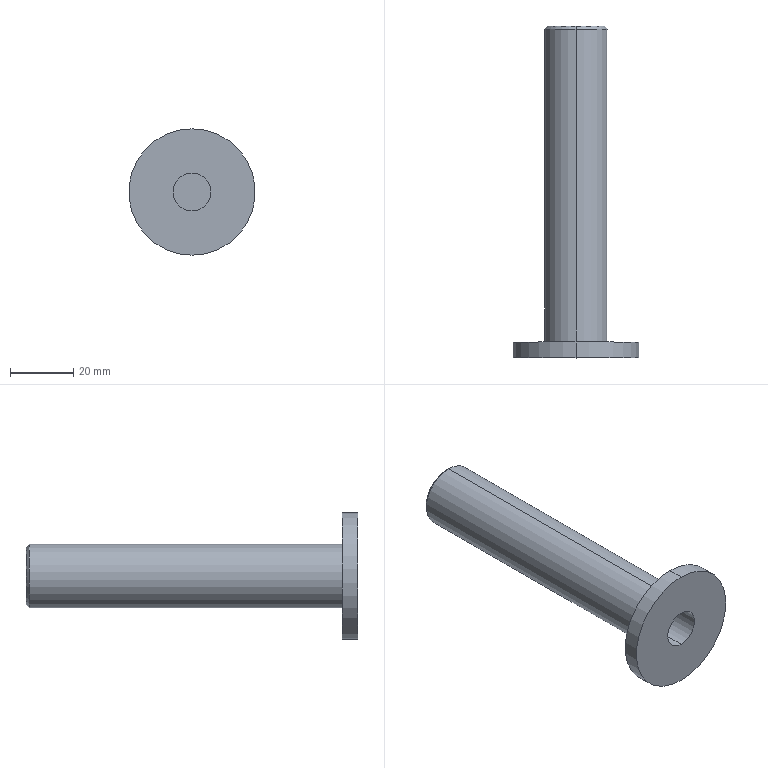Part | STEP file | Guide wheel mechanism revised.sldasm-Part-336 | 1 solid | 12 faces | box 40 x 105 x 40 mm | volume 36538 mm3 | cylinder 6 | plane 4 | cone 2 | commonest cylinder face diameters 12 x2 20 x2 40 x2
STEP:
#1=CARTESIAN_POINT('',(0.,10.,6.));
#2=VERTEX_POINT('',#1);
#3=CARTESIAN_POINT('',(0.,10.,-6.));
#4=VERTEX_POINT('',#3);
#5=CARTESIAN_POINT('',(0.,10.,0.));
#6=DIRECTION('',(0.,-1.,0.));
#7=DIRECTION('',(0.,0.,-1.));
#8=AXIS2_PLACEMENT_3D('',#5,#6,#7);
#9=CIRCLE('',#8,6.);
#10=EDGE_CURVE('',#2,#4,#9,.T.);
#11=ORIENTED_EDGE('',*,*,#10,.F.);
#12=CARTESIAN_POINT('',(0.,0.,6.));
#13=VERTEX_POINT('',#12);
#14=CARTESIAN_POINT('',(0.,10.,6.));
#15=DIRECTION('',(0.,-1.,0.));
#16=VECTOR('',#15,1000.);
#17=LINE('',#14,#16);
#18=EDGE_CURVE('',#2,#13,#17,.T.);
#19=ORIENTED_EDGE('',*,*,#18,.T.);
#20=CARTESIAN_POINT('',(0.,0.,-6.));
#21=VERTEX_POINT('',#20);
#22=CARTESIAN_POINT('',(0.,0.,0.));
#23=DIRECTION('',(0.,-1.,0.));
#24=DIRECTION('',(0.,0.,-1.));
#25=AXIS2_PLACEMENT_3D('',#22,#23,#24);
#26=CIRCLE('',#25,6.);
#27=EDGE_CURVE('',#13,#21,#26,.T.);
#28=ORIENTED_EDGE('',*,*,#27,.T.);
#29=CARTESIAN_POINT('',(0.,10.,-6.));
#30=DIRECTION('',(0.,-1.,0.));
#31=VECTOR('',#30,1000.);
#32=LINE('',#29,#31);
#33=EDGE_CURVE('',#4,#21,#32,.T.);
#34=ORIENTED_EDGE('',*,*,#33,.F.);
#35=EDGE_LOOP('',(#11,#19,#28,#34));
#36=FACE_OUTER_BOUND('',#35,.T.);
#37=CARTESIAN_POINT('',(0.,10.,0.));
#38=DIRECTION('',(0.,-1.,0.));
#39=DIRECTION('',(0.,0.,-1.));
#40=AXIS2_PLACEMENT_3D('',#37,#38,#39);
#41=CYLINDRICAL_SURFACE('',#40,6.);
#42=ADVANCED_FACE('',(#36),#41,.F.);
#43=CARTESIAN_POINT('',(0.,5.,-20.));
#44=VERTEX_POINT('',#43);
#45=CARTESIAN_POINT('',(0.,5.,20.));
#46=VERTEX_POINT('',#45);
#47=CARTESIAN_POINT('',(0.,5.,0.));
#48=DIRECTION('',(0.,-1.,0.));
#49=DIRECTION('',(0.,0.,-1.));
#50=AXIS2_PLACEMENT_3D('',#47,#48,#49);
#51=CIRCLE('',#50,20.);
#52=EDGE_CURVE('',#44,#46,#51,.T.);
#53=ORIENTED_EDGE('',*,*,#52,.T.);
#54=CARTESIAN_POINT('',(0.,0.,20.));
#55=VERTEX_POINT('',#54);
#56=CARTESIAN_POINT('',(0.,10.,20.));
#57=DIRECTION('',(0.,-1.,0.));
#58=VECTOR('',#57,1000.);
#59=LINE('',#56,#58);
#60=EDGE_CURVE('',#46,#55,#59,.T.);
#61=ORIENTED_EDGE('',*,*,#60,.T.);
#62=CARTESIAN_POINT('',(0.,0.,-20.));
#63=VERTEX_POINT('',#62);
#64=CARTESIAN_POINT('',(0.,0.,0.));
#65=DIRECTION('',(0.,-1.,0.));
#66=DIRECTION('',(0.,0.,-1.));
#67=AXIS2_PLACEMENT_3D('',#64,#65,#66);
#68=CIRCLE('',#67,20.);
#69=EDGE_CURVE('',#63,#55,#68,.T.);
#70=ORIENTED_EDGE('',*,*,#69,.F.);
#71=CARTESIAN_POINT('',(0.,10.,-20.));
#72=DIRECTION('',(0.,-1.,0.));
#73=VECTOR('',#72,1000.);
#74=LINE('',#71,#73);
#75=EDGE_CURVE('',#44,#63,#74,.T.);
#76=ORIENTED_EDGE('',*,*,#75,.F.);
#77=EDGE_LOOP('',(#53,#61,#70,#76));
#78=FACE_OUTER_BOUND('',#77,.T.);
#79=CARTESIAN_POINT('',(0.,10.,0.));
#80=DIRECTION('',(0.,-1.,0.));
#81=DIRECTION('',(0.,0.,-1.));
#82=AXIS2_PLACEMENT_3D('',#79,#80,#81);
#83=CYLINDRICAL_SURFACE('',#82,20.);
#84=ADVANCED_FACE('',(#78),#83,.T.);
#85=CARTESIAN_POINT('',(0.,104.,-10.));
#86=VERTEX_POINT('',#85);
#87=CARTESIAN_POINT('',(0.,104.,10.));
#88=VERTEX_POINT('',#87);
#89=CARTESIAN_POINT('',(0.,104.,0.));
#90=DIRECTION('',(0.,-1.,0.));
#91=DIRECTION('',(0.,0.,-1.));
#92=AXIS2_PLACEMENT_3D('',#89,#90,#91);
#93=CIRCLE('',#92,10.);
#94=EDGE_CURVE('',#86,#88,#93,.T.);
#95=ORIENTED_EDGE('',*,*,#94,.T.);
#96=CARTESIAN_POINT('',(0.,5.,10.));
#97=VERTEX_POINT('',#96);
#98=CARTESIAN_POINT('',(0.,10.,10.));
#99=DIRECTION('',(0.,-1.,0.));
#100=VECTOR('',#99,1000.);
#101=LINE('',#98,#100);
#102=EDGE_CURVE('',#88,#97,#101,.T.);
#103=ORIENTED_EDGE('',*,*,#102,.T.);
#104=CARTESIAN_POINT('',(0.,5.,-10.));
#105=VERTEX_POINT('',#104);
#106=CARTESIAN_POINT('',(0.,5.,0.));
#107=DIRECTION('',(0.,-1.,0.));
#108=DIRECTION('',(0.,0.,-1.));
#109=AXIS2_PLACEMENT_3D('',#106,#107,#108);
#110=CIRCLE('',#109,10.);
#111=EDGE_CURVE('',#105,#97,#110,.T.);
#112=ORIENTED_EDGE('',*,*,#111,.F.);
#113=CARTESIAN_POINT('',(0.,10.,-10.));
#114=DIRECTION('',(0.,-1.,0.));
#115=VECTOR('',#114,1000.);
#116=LINE('',#113,#115);
#117=EDGE_CURVE('',#86,#105,#116,.T.);
#118=ORIENTED_EDGE('',*,*,#117,.F.);
#119=EDGE_LOOP('',(#95,#103,#112,#118));
#120=FACE_OUTER_BOUND('',#119,.T.);
#121=CARTESIAN_POINT('',(0.,10.,0.));
#122=DIRECTION('',(0.,-1.,0.));
#123=DIRECTION('',(0.,0.,-1.));
#124=AXIS2_PLACEMENT_3D('',#121,#122,#123);
#125=CYLINDRICAL_SURFACE('',#124,10.);
#126=ADVANCED_FACE('',(#120),#125,.T.);
#127=CARTESIAN_POINT('',(0.,105.,-9.));
#128=VERTEX_POINT('',#127);
#129=CARTESIAN_POINT('',(0.,105.,9.));
#130=VERTEX_POINT('',#129);
#131=CARTESIAN_POINT('',(0.,105.,0.));
#132=DIRECTION('',(0.,-1.,0.));
#133=DIRECTION('',(0.,0.,-1.));
#134=AXIS2_PLACEMENT_3D('',#131,#132,#133);
#135=CIRCLE('',#134,9.);
#136=EDGE_CURVE('',#128,#130,#135,.T.);
#137=ORIENTED_EDGE('',*,*,#136,.T.);
#138=CARTESIAN_POINT('',(0.,104.,10.));
#139=DIRECTION('',(0.,-0.7071,0.7071));
#140=VECTOR('',#139,1000.);
#141=LINE('',#138,#140);
#142=EDGE_CURVE('',#130,#88,#141,.T.);
#143=ORIENTED_EDGE('',*,*,#142,.T.);
#144=ORIENTED_EDGE('',*,*,#94,.F.);
#145=CARTESIAN_POINT('',(0.,104.,-10.));
#146=DIRECTION('',(0.,-0.7071,-0.7071));
#147=VECTOR('',#146,1000.);
#148=LINE('',#145,#147);
#149=EDGE_CURVE('',#128,#86,#148,.T.);
#150=ORIENTED_EDGE('',*,*,#149,.F.);
#151=EDGE_LOOP('',(#137,#143,#144,#150));
#152=FACE_OUTER_BOUND('',#151,.T.);
#153=CARTESIAN_POINT('',(0.,104.,0.));
#154=DIRECTION('',(0.,-1.,0.));
#155=DIRECTION('',(0.,0.,-1.));
#156=AXIS2_PLACEMENT_3D('',#153,#154,#155);
#157=CONICAL_SURFACE('',#156,10.,0.7854);
#158=ADVANCED_FACE('',(#152),#157,.T.);
#159=CARTESIAN_POINT('',(0.,10.,0.));
#160=DIRECTION('',(0.,-1.,0.));
#161=DIRECTION('',(0.,0.,-1.));
#162=AXIS2_PLACEMENT_3D('',#159,#160,#161);
#163=CIRCLE('',#162,6.);
#164=EDGE_CURVE('',#4,#2,#163,.T.);
#165=ORIENTED_EDGE('',*,*,#164,.T.);
#166=ORIENTED_EDGE('',*,*,#10,.T.);
#167=EDGE_LOOP('',(#165,#166));
#168=FACE_OUTER_BOUND('',#167,.T.);
#169=CARTESIAN_POINT('',(0.,10.,0.));
#170=DIRECTION('',(0.,-1.,0.));
#171=DIRECTION('',(0.,0.,-1.));
#172=AXIS2_PLACEMENT_3D('',#169,#170,#171);
#173=PLANE('',#172);
#174=ADVANCED_FACE('',(#168),#173,.T.);
#175=ORIENTED_EDGE('',*,*,#136,.F.);
#176=CARTESIAN_POINT('',(0.,105.,0.));
#177=DIRECTION('',(0.,-1.,0.));
#178=DIRECTION('',(0.,0.,-1.));
#179=AXIS2_PLACEMENT_3D('',#176,#177,#178);
#180=CIRCLE('',#179,9.);
#181=EDGE_CURVE('',#130,#128,#180,.T.);
#182=ORIENTED_EDGE('',*,*,#181,.F.);
#183=EDGE_LOOP('',(#175,#182));
#184=FACE_OUTER_BOUND('',#183,.T.);
#185=CARTESIAN_POINT('',(0.,105.,0.));
#186=DIRECTION('',(0.,1.,0.));
#187=DIRECTION('',(0.,0.,1.));
#188=AXIS2_PLACEMENT_3D('',#185,#186,#187);
#189=PLANE('',#188);
#190=ADVANCED_FACE('',(#184),#189,.T.);
#191=ORIENTED_EDGE('',*,*,#142,.F.);
#192=ORIENTED_EDGE('',*,*,#181,.T.);
#193=ORIENTED_EDGE('',*,*,#149,.T.);
#194=CARTESIAN_POINT('',(0.,104.,0.));
#195=DIRECTION('',(0.,-1.,0.));
#196=DIRECTION('',(0.,0.,-1.));
#197=AXIS2_PLACEMENT_3D('',#194,#195,#196);
#198=CIRCLE('',#197,10.);
#199=EDGE_CURVE('',#88,#86,#198,.T.);
#200=ORIENTED_EDGE('',*,*,#199,.F.);
#201=EDGE_LOOP('',(#191,#192,#193,#200));
#202=FACE_OUTER_BOUND('',#201,.T.);
#203=CARTESIAN_POINT('',(0.,104.,0.));
#204=DIRECTION('',(0.,-1.,0.));
#205=DIRECTION('',(0.,0.,-1.));
#206=AXIS2_PLACEMENT_3D('',#203,#204,#205);
#207=CONICAL_SURFACE('',#206,10.,0.7854);
#208=ADVANCED_FACE('',(#202),#207,.T.);
#209=ORIENTED_EDGE('',*,*,#102,.F.);
#210=ORIENTED_EDGE('',*,*,#199,.T.);
#211=ORIENTED_EDGE('',*,*,#117,.T.);
#212=CARTESIAN_POINT('',(0.,5.,0.));
#213=DIRECTION('',(0.,-1.,0.));
#214=DIRECTION('',(0.,0.,-1.));
#215=AXIS2_PLACEMENT_3D('',#212,#213,#214);
#216=CIRCLE('',#215,10.);
#217=EDGE_CURVE('',#97,#105,#216,.T.);
#218=ORIENTED_EDGE('',*,*,#217,.F.);
#219=EDGE_LOOP('',(#209,#210,#211,#218));
#220=FACE_OUTER_BOUND('',#219,.T.);
#221=CARTESIAN_POINT('',(0.,10.,0.));
#222=DIRECTION('',(0.,-1.,0.));
#223=DIRECTION('',(0.,0.,-1.));
#224=AXIS2_PLACEMENT_3D('',#221,#222,#223);
#225=CYLINDRICAL_SURFACE('',#224,10.);
#226=ADVANCED_FACE('',(#220),#225,.T.);
#227=ORIENTED_EDGE('',*,*,#111,.T.);
#228=ORIENTED_EDGE('',*,*,#217,.T.);
#229=EDGE_LOOP('',(#227,#228));
#230=FACE_BOUND('',#229,.T.);
#231=ORIENTED_EDGE('',*,*,#52,.F.);
#232=CARTESIAN_POINT('',(0.,5.,0.));
#233=DIRECTION('',(0.,-1.,0.));
#234=DIRECTION('',(0.,0.,-1.));
#235=AXIS2_PLACEMENT_3D('',#232,#233,#234);
#236=CIRCLE('',#235,20.);
#237=EDGE_CURVE('',#46,#44,#236,.T.);
#238=ORIENTED_EDGE('',*,*,#237,.F.);
#239=EDGE_LOOP('',(#231,#238));
#240=FACE_OUTER_BOUND('',#239,.T.);
#241=CARTESIAN_POINT('',(10.,5.,0.));
#242=DIRECTION('',(0.,1.,0.));
#243=DIRECTION('',(0.,0.,1.));
#244=AXIS2_PLACEMENT_3D('',#241,#242,#243);
#245=PLANE('',#244);
#246=ADVANCED_FACE('',(#230,#240),#245,.T.);
#247=ORIENTED_EDGE('',*,*,#60,.F.);
#248=ORIENTED_EDGE('',*,*,#237,.T.);
#249=ORIENTED_EDGE('',*,*,#75,.T.);
#250=CARTESIAN_POINT('',(0.,0.,0.));
#251=DIRECTION('',(0.,-1.,0.));
#252=DIRECTION('',(0.,0.,-1.));
#253=AXIS2_PLACEMENT_3D('',#250,#251,#252);
#254=CIRCLE('',#253,20.);
#255=EDGE_CURVE('',#55,#63,#254,.T.);
#256=ORIENTED_EDGE('',*,*,#255,.F.);
#257=EDGE_LOOP('',(#247,#248,#249,#256));
#258=FACE_OUTER_BOUND('',#257,.T.);
#259=CARTESIAN_POINT('',(0.,10.,0.));
#260=DIRECTION('',(0.,-1.,0.));
#261=DIRECTION('',(0.,0.,-1.));
#262=AXIS2_PLACEMENT_3D('',#259,#260,#261);
#263=CYLINDRICAL_SURFACE('',#262,20.);
#264=ADVANCED_FACE('',(#258),#263,.T.);
#265=ORIENTED_EDGE('',*,*,#69,.T.);
#266=ORIENTED_EDGE('',*,*,#255,.T.);
#267=EDGE_LOOP('',(#265,#266));
#268=FACE_OUTER_BOUND('',#267,.T.);
#269=CARTESIAN_POINT('',(0.,0.,0.));
#270=DIRECTION('',(0.,-1.,0.));
#271=DIRECTION('',(0.,0.,-1.));
#272=AXIS2_PLACEMENT_3D('',#269,#270,#271);
#273=CIRCLE('',#272,6.);
#274=EDGE_CURVE('',#21,#13,#273,.T.);
#275=ORIENTED_EDGE('',*,*,#274,.F.);
#276=ORIENTED_EDGE('',*,*,#27,.F.);
#277=EDGE_LOOP('',(#275,#276));
#278=FACE_BOUND('',#277,.T.);
#279=CARTESIAN_POINT('',(20.,0.,0.));
#280=DIRECTION('',(0.,-1.,0.));
#281=DIRECTION('',(0.,0.,-1.));
#282=AXIS2_PLACEMENT_3D('',#279,#280,#281);
#283=PLANE('',#282);
#284=ADVANCED_FACE('',(#268,#278),#283,.T.);
#285=ORIENTED_EDGE('',*,*,#18,.F.);
#286=ORIENTED_EDGE('',*,*,#164,.F.);
#287=ORIENTED_EDGE('',*,*,#33,.T.);
#288=ORIENTED_EDGE('',*,*,#274,.T.);
#289=EDGE_LOOP('',(#285,#286,#287,#288));
#290=FACE_OUTER_BOUND('',#289,.T.);
#291=CARTESIAN_POINT('',(0.,10.,0.));
#292=DIRECTION('',(0.,-1.,0.));
#293=DIRECTION('',(0.,0.,-1.));
#294=AXIS2_PLACEMENT_3D('',#291,#292,#293);
#295=CYLINDRICAL_SURFACE('',#294,6.);
#296=ADVANCED_FACE('',(#290),#295,.F.);
#297=CLOSED_SHELL('',(#42,#84,#126,#158,#174,#190,#208,#226,#246,#264,#284,#296));
#298=MANIFOLD_SOLID_BREP('',#297);
#299=CARTESIAN_POINT('',(0.,0.,0.));
#300=DIRECTION('',(0.,0.,1.));
#301=DIRECTION('',(1.,0.,0.));
#302=AXIS2_PLACEMENT_3D('',#299,#300,#301);
#303=(LENGTH_UNIT()NAMED_UNIT(*)SI_UNIT(.MILLI.,.METRE.));
#304=UNCERTAINTY_MEASURE_WITH_UNIT(LENGTH_MEASURE(0.00001),#303,'','');
#305=(NAMED_UNIT(*)PLANE_ANGLE_UNIT()SI_UNIT($,.RADIAN.));
#306=(NAMED_UNIT(*)SI_UNIT($,.STERADIAN.)SOLID_ANGLE_UNIT());
#307=(GEOMETRIC_REPRESENTATION_CONTEXT(3)GLOBAL_UNCERTAINTY_ASSIGNED_CONTEXT((#304))GLOBAL_UNIT_ASSIGNED_CONTEXT((#303,#305,#306))REPRESENTATION_CONTEXT('',''));
#308=ADVANCED_BREP_SHAPE_REPRESENTATION('',(#298,#302),#307);